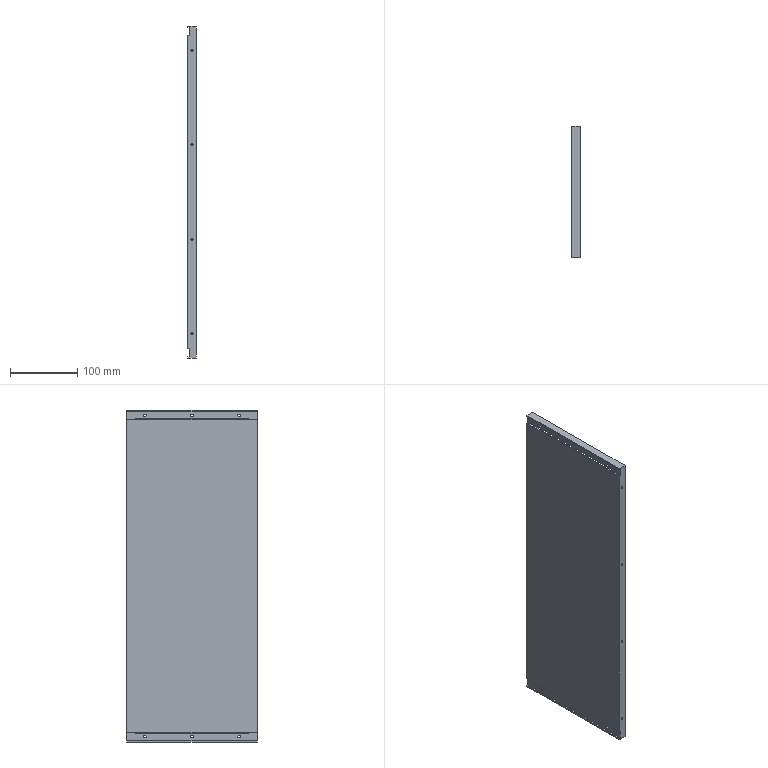Part | SolidWorks | features ICE 6, MirrorPattern 3, Extrusion 1, Fillet 1, LPattern 1 | 1 solid | 252 faces | box 12 x 194 x 493 mm | volume 496868 mm3 | plane 138 | cylinder 114 | commonest cylinder face diameters 3 x86 4 x12 6 x12 10 x4